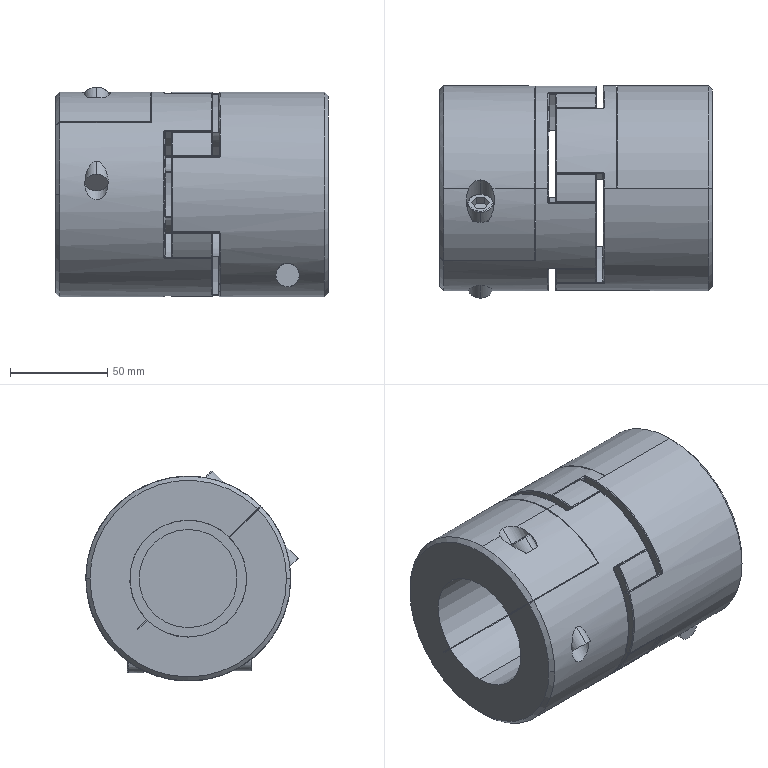Part | STEP file | LYCA jaw coupling [LYCA-105140]_LYCA-105140 | 3 solids | 407 faces | box 140 x 108.875 x 107.681 mm | volume 781609 mm3 | spline 212 | cylinder 135 | plane 55 | cone 5 | commonest cylinder face diameters 0.84 x58 63 x36 105 x13 12 x10 50.4 x4 60 x4